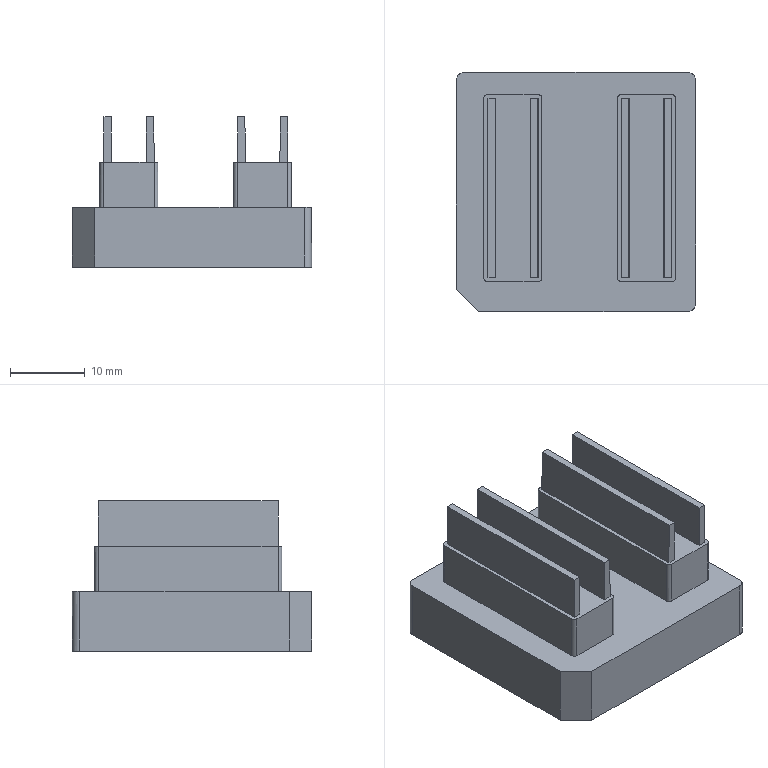NC program | PowerMill | posted with a generic post | part box 32 x 32 x 20.109 mm
Lines 1 to 1024 of 124326:
%
O0001
N104 ( POWERMILL CB  : 2026004.0)
N105 ( POST VER      : 2026.0.0.5161)
N106 ( OPTION FILE   : FANUC)
N107 ( OUTPUT WORKPLANE : WORLD)
N108 (  )
N109 ( TOOL LIST )
N110 (---------------------------------------)
N111 ( NO. | ID        | DIA.| TIP RAD|LENGTH)
N112 (---------------------------------------)
N113 (    1|D10C_1_1_1 |10.0 |  0.0   |75.56 )
N114 (   10|D3_1_1     | 3.0 |  0.0   |67.28 )
N115 (    3|D10_1_1_1  |10.0 |  0.0   |75.28 )
N116 (   10|D3_2_1     | 3.0 |  0.0   |61.32 )
N117 (   13|TEXT_D4_1_1| 4.0 |  0.3   |67.36 )
N118 (---------------------------------------)
N119 (  )
N120 ( NUMBER OF TOOLPATHS: 11.0 )
N121 ( ESTIMATED PROGRAM DURATION: 0 HOURS 28 MIN 3 SEC)
N122 (  )
N123 G00 G21 G80 G40 G17
N124 G90
N125 G54
N126 G53 Z0.0
N127 (---------------)
N128 ( START TOOLPATH : 精公开粗01-扫面平行-D10C )
N129 (---------------)
N130 ( TOOL NO.    :1 )
N131 ( TOOL TYPE   : ENDMILL)
N132 ( TOOL ID     : D10C_1_1_1)
N133 ( TOOL DIA    : 10.0 LENGTH 75.56)
N134 T1
N135 M6
N136 S8000 M03
N137 G00 G90 X0.0 Y0.0
N138 G43 Z10.2 H1
N139
N140 G05 P10000 R4
N141 X23.78 Y18.78
N142 Z1.129
N143 G01 Z-0.071 F6000.0
N144 X18.78 F10000.0
N145 X-18.78
N146 Y13.4143
N147 X18.78
N148 Y8.0486
N149 X-18.78
N150 Y2.6829
N151 X18.78
N152 Y-2.6829
N153 X-18.78
N154 Y-8.0486
N155 X18.78
N156 Y-13.4143
N157 X-18.78
N158 Y-18.78
N159 X18.78
N160 X23.78
N161 G00 Z10.2
N162 G05 P0
N163 (---------------)
N164 ( END TOOLPATH : 精公开粗01-扫面平行-D10C )
N165 (---------------)
N166 ( START TOOLPATH : 精公开粗01-外形偏置-D10C )
N167 (---------------)
N168 G00 X0.5 Y0.5 Z9.879
N169 G05 P10000 R4
N170 X1.5532 Y26.066
N171 Z0.7009
N172 G01 Z-0.4991 F6000.0
N173 Y25.5385 F10000.0
N174 G03 X6.3007 Y20.791 I4.7475 J0.0
N175 G01 X20.109
N176 G02 X21.109 Y19.791 I0.0 J-1.0
N177 G01 Y-18.791
N178 G02 X20.109 Y-19.791 I-1.0 J0.0
N179 G01 X-19.109
N180 G02 X-20.109 Y-18.791 I0.0 J1.0
N181 G01 Y19.791
N182 G02 X-19.109 Y20.791 I1.0 J0.0
N183 G01 X6.3007
N184 Y17.7935
N185 X7.0741
N186 X7.8476 Y17.7374
N187 X8.621 Y17.5636
N188 X9.2558 Y17.3098
N189 G03 X9.6337 Y17.3126 I0.1856 J0.4643
N190 G01 X10.1205 Y17.5154
N191 X10.9413 Y17.7207
N192 X11.7147 Y17.7926
N193 X13.2615 Y17.7714
N194 X14.035 Y17.642
N195 X14.8084 Y17.388
N196 X15.5818 Y16.9875
N197 X15.9412 Y16.742
N198 X16.3552 Y16.3946
N199 X16.7718 Y15.9685
N200 X17.1287 Y15.5052
N201 X17.3274 Y15.1951
N202 X17.7023 Y14.4217
N203 X17.9021 Y13.7916
N204 X18.0463 Y12.8748
N205 X18.0563 Y12.1014
N206 Y-11.1014
N207 X18.0463 Y-11.8748
N208 X17.9352 Y-12.6483
N209 X17.7023 Y-13.4217
N210 X17.3274 Y-14.1951
N211 X17.1287 Y-14.5064
N212 X16.7718 Y-14.9685
N213 X16.3552 Y-15.3962
N214 X15.9412 Y-15.742
N215 X15.5818 Y-15.9875
N216 X14.8084 Y-16.3878
N217 X14.467 Y-16.5154
N218 X14.035 Y-16.6418
N219 X13.2615 Y-16.7714
N220 X11.7147 Y-16.7926
N221 X10.9413 Y-16.7185
N222 X10.1678 Y-16.5302
N223 X9.6371 Y-16.3125
N224 G03 X9.2557 Y-16.3133 I-0.1897 J-0.4626
N225 G01 X8.7689 Y-16.5154
N226 X7.8476 Y-16.7374
N227 X7.0741 Y-16.7935
N228 X6.3007
N229 X5.5273 Y-16.7596
N230 X4.7538 Y-16.6157
N231 X4.422 Y-16.5154
N232 X3.9804 Y-16.3439
N233 X3.207 Y-15.9183
N234 X2.9505 Y-15.742
N235 X2.4336 Y-15.3013
N236 X2.1225 Y-14.9685
N237 X1.6601 Y-14.3516
N238 X1.1893 Y-13.4217
N239 X0.9577 Y-12.6483
N240 X0.8867 Y-12.2714
N241 X0.8468 Y-11.8748
N242 X0.832 Y-11.1014
N243 Y12.1014
N244 X0.8341 Y12.2088
N245 X0.1665 Y12.1981
N246 X0.168 Y12.1014
N247 Y-11.1014
N248 X0.1556 Y-11.8748
N249 X0.0443 Y-12.6483
N250 X-0.1889 Y-13.4217
N251 X-0.5637 Y-14.1951
N252 X-1.1194 Y-14.9685
N253 X-1.4336 Y-15.3013
N254 X-1.9524 Y-15.742
N255 X-2.207 Y-15.9183
N256 X-2.9804 Y-16.3439
N257 X-3.421 Y-16.5154
N258 X-3.7538 Y-16.6157
N259 X-4.5273 Y-16.7596
N260 X-5.3007 Y-16.7935
N261 X-6.0741
N262 X-6.8476 Y-16.7374
N263 X-7.621 Y-16.5636
N264 X-8.2575 Y-16.3091
N265 G03 X-8.6329 Y-16.3108 I-0.1857 J-0.4643
N266 G01 X-9.1678 Y-16.5302
N267 X-9.9413 Y-16.7185
N268 X-10.7147 Y-16.7926
N269 X-12.2615 Y-16.7714
N270 X-13.035 Y-16.6418
N271 X-13.47 Y-16.5154
N272 X-13.8084 Y-16.3878
N273 X-14.5818 Y-15.9875
N274 X-14.9391 Y-15.742
N275 X-15.3552 Y-15.3962
N276 X-15.7706 Y-14.9685
N277 X-16.1287 Y-14.5064
N278 X-16.3274 Y-14.1951
N279 X-16.7019 Y-13.4217
N280 X-16.9021 Y-12.7918
N281 X-17.0464 Y-11.8748
N282 X-17.059 Y-11.1014
N283 Y12.1014
N284 X-17.0464 Y12.8748
N285 X-16.9352 Y13.6483
N286 X-16.7019 Y14.4217
N287 X-16.3274 Y15.1951
N288 X-16.1287 Y15.5052
N289 X-15.7706 Y15.9685
N290 X-15.3552 Y16.3946
N291 X-14.9391 Y16.742
N292 X-14.5818 Y16.9875
N293 X-13.8084 Y17.388
N294 X-13.47 Y17.5154
N295 X-13.035 Y17.642
N296 X-12.2615 Y17.7714
N297 X-10.7147 Y17.7926
N298 X-9.9413 Y17.7207
N299 X-9.1678 Y17.5302
N300 X-8.6369 Y17.3124
N301 G03 X-8.2556 Y17.3131 I0.1898 J0.4626
N302 G01 X-7.7679 Y17.5154
N303 X-6.8476 Y17.7374
N304 X-6.0741 Y17.7935
N305 X-5.3007
N306 X-4.5273 Y17.7596
N307 X-3.7538 Y17.6157
N308 X-3.421 Y17.5154
N309 X-2.9804 Y17.343
N310 X-2.207 Y16.9225
N311 X-1.9525 Y16.742
N312 X-1.4336 Y16.2981
N313 X-1.1194 Y15.9685
N314 X-0.5637 Y15.1951
N315 X-0.1889 Y14.4217
N316 X0.0443 Y13.6483
N317 X0.1556 Y12.8748
N318 X0.1665 Y12.1981
N319 X0.8341 Y12.2088
N320 X0.8468 Y12.8748
N321 X0.8867 Y13.2713
N322 X0.9577 Y13.6483
N323 X1.1893 Y14.4217
N324 X1.5642 Y15.1951
N325 X2.1225 Y15.9685
N326 X2.4336 Y16.2981
N327 X2.9505 Y16.742
N328 X3.207 Y16.9225
N329 X3.9804 Y17.343
N330 X4.422 Y17.5154
N331 X4.7538 Y17.6157
N332 X5.5273 Y17.7596
N333 X6.3007 Y17.7935
N334 Y20.791
N335 G00 Z3.3228
N336 G01 X1.5532 Y26.066
N337 G00 Z0.3228
N338 G01 Z-0.8772 F6000.0
N339 Y25.5385 F10000.0
N340 G03 X6.3007 Y20.791 I4.7475 J0.0
N341 G01 X20.109
N342 G02 X21.109 Y19.791 I0.0 J-1.0
N343 G01 Y-18.791
N344 G02 X20.109 Y-19.791 I-1.0 J0.0
N345 G01 X-19.109
N346 G02 X-20.109 Y-18.791 I0.0 J1.0
N347 G01 Y19.791
N348 G02 X-19.109 Y20.791 I1.0 J0.0
N349 G01 X6.3007
N350 Y17.7935
N351 X7.0741
N352 X7.8476 Y17.7379
N353 X8.621 Y17.5646
N354 X9.2575 Y17.3106
N355 G03 X9.6328 Y17.3125 I0.1853 J0.4644
N356 G01 X9.6987 Y17.3396
N357 X10.1205 Y17.5153
N358 X10.1358 Y17.5192
N359 X10.1678 Y17.5323
N360 X10.9413 Y17.7219
N361 X11.7147 Y17.7927
N362 X13.2615 Y17.7717
N363 X14.035 Y17.6428
N364 X14.4735 Y17.5154
N365 X14.8084 Y17.3894
N366 X15.5818 Y16.9901
N367 X15.9445 Y16.742
N368 X16.3552 Y16.4012
N369 X16.7751 Y15.9685
N370 X17.1287 Y15.5116
N371 X17.3308 Y15.1951
N372 X17.7056 Y14.4217
N373 X17.9021 Y13.8045
N374 X18.0501 Y12.8748
N375 X18.0615 Y12.1014
N376 Y-11.1014
N377 X18.0501 Y-11.8748
N378 X17.9391 Y-12.6483
N379 X17.7056 Y-13.4217
N380 X17.3308 Y-14.1951
N381 X17.1287 Y-14.5116
N382 X16.7751 Y-14.9685
N383 X16.3552 Y-15.4005
N384 X15.9445 Y-15.742
N385 X15.5818 Y-15.9901
N386 X14.8084 Y-16.3894
N387 X14.4735 Y-16.5154
N388 X14.035 Y-16.6428
N389 X13.2615 Y-16.7717
N390 X11.7147 Y-16.7927
N391 X10.9413 Y-16.7215
N392 X10.1678 Y-16.5323
N393 X9.6375 Y-16.3145
N394 G03 X9.2555 Y-16.3153 I-0.19 J-0.4625
N395 G01 X8.7743 Y-16.5154
N396 X7.8476 Y-16.7379
N397 X7.0741 Y-16.7935
N398 X6.3007
N399 X5.5273 Y-16.761
N400 X4.7538 Y-16.6167
N401 X4.4177 Y-16.5154
N402 X3.9804 Y-16.3456
N403 X3.207 Y-15.9247
N404 X2.9467 Y-15.742
N405 X2.4336 Y-15.3045
N406 X2.1164 Y-14.9685
N407 X1.971 Y-14.7662
N408 X1.6602 Y-14.3516
N409 X1.63 Y-14.292
N410 X1.5604 Y-14.1951
N411 X1.1856 Y-13.4217
N412 X0.9531 Y-12.6483
N413 X0.8867 Y-12.294
N414 X0.842 Y-11.8748
N415 X0.8287 Y-11.1014
N416 Y12.1014
N417 X0.1713
N418 Y-11.1014
N419 X0.1589 Y-11.8748
N420 X0.0479 Y-12.6483
N421 X-0.1856 Y-13.4217
N422 X-0.5604 Y-14.1951
N423 X-1.1161 Y-14.9685
N424 X-1.4336 Y-15.3045
N425 X-1.9476 Y-15.742
N426 X-2.207 Y-15.9247
N427 X-2.9804 Y-16.3456
N428 X-3.4177 Y-16.5154
N429 X-3.7538 Y-16.6167
N430 X-4.5273 Y-16.761
N431 X-5.3007 Y-16.7935
N432 X-6.0741
N433 X-6.8476 Y-16.7379
N434 X-7.621 Y-16.5646
N435 X-8.2575 Y-16.3106
N436 G03 X-8.6328 Y-16.3125 I-0.1853 J-0.4644
N437 G01 X-9.1678 Y-16.5323
N438 X-9.9413 Y-16.7215
N439 X-10.7147 Y-16.7927
N440 X-12.2615 Y-16.7717
N441 X-13.035 Y-16.6428
N442 X-13.4735 Y-16.5154
N443 X-13.8084 Y-16.3894
N444 X-14.5818 Y-15.9901
N445 X-14.9445 Y-15.742
N446 X-15.3552 Y-15.4005
N447 X-15.7751 Y-14.9685
N448 X-16.1287 Y-14.5116
N449 X-16.3308 Y-14.1951
N450 X-16.7056 Y-13.4217
N451 X-16.9021 Y-12.8046
N452 X-17.0501 Y-11.8748
N453 X-17.0625 Y-11.1014
N454 Y12.1014
N455 X-17.0501 Y12.8748
N456 X-16.9391 Y13.6483
N457 X-16.7056 Y14.4217
N458 X-16.3308 Y15.1951
N459 X-16.1287 Y15.5116
N460 X-15.7751 Y15.9685
N461 X-15.3552 Y16.4012
N462 X-14.9445 Y16.742
N463 X-14.5818 Y16.9901
N464 X-13.8084 Y17.3894
N465 X-13.4735 Y17.5154
N466 X-13.035 Y17.6428
N467 X-12.2615 Y17.7717
N468 X-10.7147 Y17.7927
N469 X-9.9413 Y17.7219
N470 X-9.1678 Y17.5323
N471 X-8.6375 Y17.3144
N472 G03 X-8.2555 Y17.3153 I0.19 J0.4625
N473 G01 X-7.7743 Y17.5154
N474 X-6.8476 Y17.7379
N475 X-6.0741 Y17.7935
N476 X-5.3007
N477 X-4.5273 Y17.761
N478 X-3.7538 Y17.6167
N479 X-3.4177 Y17.5154
N480 X-2.9804 Y17.3456
N481 X-2.207 Y16.9247
N482 X-1.9476 Y16.742
N483 X-1.4336 Y16.3045
N484 X-1.1161 Y15.9685
N485 X-0.5604 Y15.1951
N486 X-0.1856 Y14.4217
N487 X0.0479 Y13.6483
N488 X0.1589 Y12.8748
N489 X0.1713 Y12.1014
N490 X0.8287
N491 X0.842 Y12.8748
N492 X0.8867 Y13.293
N493 X0.9531 Y13.6483
N494 X1.1856 Y14.4217
N495 X1.5604 Y15.1951
N496 X2.1164 Y15.9685
N497 X2.4336 Y16.3045
N498 X2.9467 Y16.742
N499 X3.207 Y16.9247
N500 X3.9804 Y17.3456
N501 X4.4177 Y17.5154
N502 X4.7538 Y17.6167
N503 X5.5273 Y17.761
N504 X6.3007 Y17.7935
N505 Y20.791
N506 G00 Z2.9447
N507 G01 X1.5532 Y26.066
N508 G00 Z-0.0553
N509 G01 Z-1.2553 F6000.0
N510 Y25.5385 F10000.0
N511 G03 X6.3007 Y20.791 I4.7475 J0.0
N512 G01 X20.109
N513 G02 X21.109 Y19.791 I0.0 J-1.0
N514 G01 Y-18.791
N515 G02 X20.109 Y-19.791 I-1.0 J0.0
N516 G01 X-19.109
N517 G02 X-20.109 Y-18.791 I0.0 J1.0
N518 G01 Y19.791
N519 G02 X-19.109 Y20.791 I1.0 J0.0
N520 G01 X6.3007
N521 Y17.7935
N522 X7.0741
N523 X7.8476 Y17.7384
N524 X8.621 Y17.5656
N525 X9.2577 Y17.3121
N526 G03 X9.6323 Y17.3139 I0.185 J0.4645
N527 G01 X9.9334 Y17.4373
N528 X10.1205 Y17.5153
N529 X10.1286 Y17.5173
N530 X10.1678 Y17.5334
N531 X10.9413 Y17.7224
N532 X11.7147 Y17.7927
N533 X13.2615 Y17.772
N534 X14.035 Y17.6436
N535 X14.4768 Y17.5154
N536 X14.8084 Y17.3907
N537 X15.5818 Y16.9924
N538 X15.9478 Y16.742
N539 X16.3552 Y16.4042
N540 X16.7784 Y15.9685
N541 X17.1287 Y15.5165
N542 X17.3341 Y15.1951
N543 X17.7089 Y14.4217
N544 X17.9021 Y13.8173
N545 X18.0534 Y12.8748
N546 X18.0658 Y12.1014
N547 Y-11.1014
N548 X18.0534 Y-11.8748
N549 X17.9424 Y-12.6483
N550 X17.7089 Y-13.4217
N551 X17.3341 Y-14.1951
N552 X17.1287 Y-14.5165
N553 X16.7784 Y-14.9685
N554 X16.3552 Y-15.4042
N555 X15.9478 Y-15.742
N556 X15.5818 Y-15.9924
N557 X14.8084 Y-16.3907
N558 X14.4768 Y-16.5154
N559 X14.035 Y-16.6436
N560 X13.2615 Y-16.772
N561 X11.7147 Y-16.7927
N562 X10.9413 Y-16.7224
N563 X10.1678 Y-16.5334
N564 X9.637 Y-16.3157
N565 G03 X9.2553 Y-16.3167 I-0.1897 J-0.4627
N566 G01 X8.7776 Y-16.5154
N567 X7.8476 Y-16.7384
N568 X7.0741 Y-16.7935
N569 X6.3007
N570 X5.5273 Y-16.7617
N571 X4.7538 Y-16.6176
N572 X4.4144 Y-16.5154
N573 X3.9804 Y-16.347
N574 X3.207 Y-15.9268
N575 X2.9434 Y-15.742
N576 X2.4336 Y-15.3077
N577 X2.1128 Y-14.9685
N578 X1.8834 Y-14.6494
N579 X1.6602 Y-14.3516
N580 X1.6382 Y-14.308
N581 X1.5571 Y-14.1951
N582 X1.1823 Y-13.4217
N583 X0.9488 Y-12.6483
N584 X0.9345 Y-12.5485
N585 X0.8868 Y-12.294
N586 X0.8544 Y-11.991
N587 X0.8378 Y-11.8748
N588 X0.8254 Y-11.1014
N589 Y12.1014
N590 X0.1746
N591 Y-11.1014
N592 X0.1622 Y-11.8748
N593 X0.0512 Y-12.6483
N594 X-0.1823 Y-13.4217
N595 X-0.5571 Y-14.1951
N596 X-1.1128 Y-14.9685
N597 X-1.4336 Y-15.3077
N598 X-1.9434 Y-15.742
N599 X-2.207 Y-15.9268
N600 X-2.9804 Y-16.347
N601 X-3.4144 Y-16.5154
N602 X-3.7538 Y-16.6176
N603 X-4.5273 Y-16.7617
N604 X-5.3007 Y-16.7935
N605 X-6.0741
N606 X-6.8476 Y-16.7384
N607 X-7.621 Y-16.5656
N608 X-8.2577 Y-16.3121
N609 G03 X-8.6322 Y-16.3139 I-0.185 J-0.4645
N610 G01 X-9.1678 Y-16.5334
N611 X-9.9413 Y-16.7224
N612 X-10.7147 Y-16.7927
N613 X-12.2615 Y-16.772
N614 X-13.035 Y-16.6436
N615 X-13.4768 Y-16.5154
N616 X-13.8084 Y-16.3907
N617 X-14.5818 Y-15.9924
N618 X-14.9478 Y-15.742
N619 X-15.3552 Y-15.4042
N620 X-15.7784 Y-14.9685
N621 X-16.1287 Y-14.5165
N622 X-16.3341 Y-14.1951
N623 X-16.7089 Y-13.4217
N624 X-16.9021 Y-12.8174
N625 X-17.0534 Y-11.8748
N626 X-17.0658 Y-11.1014
N627 Y12.1014
N628 X-17.0534 Y12.8748
N629 X-16.9424 Y13.6483
N630 X-16.7089 Y14.4217
N631 X-16.3341 Y15.1951
N632 X-16.1287 Y15.5165
N633 X-15.7784 Y15.9685
N634 X-15.3552 Y16.4042
N635 X-14.9478 Y16.742
N636 X-14.5818 Y16.9924
N637 X-13.8084 Y17.3907
N638 X-13.4768 Y17.5154
N639 X-13.035 Y17.6436
N640 X-12.2615 Y17.772
N641 X-10.7147 Y17.7927
N642 X-9.9413 Y17.7224
N643 X-9.1678 Y17.5334
N644 X-8.6371 Y17.3158
N645 G03 X-8.2554 Y17.3167 I0.1897 J0.4626
N646 G01 X-7.7776 Y17.5154
N647 X-6.8476 Y17.7384
N648 X-6.0741 Y17.7935
N649 X-5.3007
N650 X-4.5273 Y17.7617
N651 X-3.7538 Y17.6176
N652 X-3.4144 Y17.5154
N653 X-2.9804 Y17.347
N654 X-2.207 Y16.9268
N655 X-1.9434 Y16.742
N656 X-1.4336 Y16.3077
N657 X-1.1128 Y15.9685
N658 X-0.5571 Y15.1951
N659 X-0.1823 Y14.4217
N660 X0.0512 Y13.6483
N661 X0.1622 Y12.8748
N662 X0.1746 Y12.1014
N663 X0.8254
N664 X0.8378 Y12.8748
N665 X0.8546 Y12.9918
N666 X0.8868 Y13.293
N667 X0.9343 Y13.5473
N668 X0.9488 Y13.6483
N669 X1.1823 Y14.4217
N670 X1.5571 Y15.1951
N671 X2.1128 Y15.9685
N672 X2.4336 Y16.3077
N673 X2.9434 Y16.742
N674 X3.207 Y16.9268
N675 X3.9804 Y17.347
N676 X4.4144 Y17.5154
N677 X4.7538 Y17.6176
N678 X5.5273 Y17.7617
N679 X6.3007 Y17.7935
N680 Y20.791
N681 G00 Z2.5666
N682 G01 X1.5532 Y26.066
N683 G00 Z-0.4334
N684 G01 Z-1.6334 F6000.0
N685 Y25.5385 F10000.0
N686 G03 X6.3007 Y20.791 I4.7475 J0.0
N687 G01 X20.109
N688 G02 X21.109 Y19.791 I0.0 J-1.0
N689 G01 Y-18.791
N690 G02 X20.109 Y-19.791 I-1.0 J0.0
N691 G01 X-19.109
N692 G02 X-20.109 Y-18.791 I0.0 J1.0
N693 G01 Y19.791
N694 G02 X-19.109 Y20.791 I1.0 J0.0
N695 G01 X6.3007
N696 Y17.7935
N697 X7.0741
N698 X7.8476 Y17.7389
N699 X8.621 Y17.5666
N700 X9.2578 Y17.3135
N701 G03 X9.6317 Y17.3153 I0.1847 J0.4647
N702 G01 X10.1074 Y17.5098
N703 X10.1205 Y17.5152
N704 X10.1212 Y17.5154
N705 X10.1678 Y17.5345
N706 X10.9413 Y17.723
N707 X11.7147 Y17.7928
N708 X13.2615 Y17.7723
N709 X14.035 Y17.6444
N710 X14.4801 Y17.5154
N711 X14.8084 Y17.3921
N712 X15.5818 Y16.9945
N713 X15.9511 Y16.742
N714 X16.3552 Y16.4072
N715 X16.7817 Y15.9685
N716 X17.1287 Y15.5212
N717 X17.3374 Y15.1951
N718 X17.7122 Y14.4217
N719 X17.9021 Y13.8302
N720 X18.0567 Y12.8748
N721 X18.0691 Y12.1014
N722 Y-11.1014
N723 X18.0567 Y-11.8748
N724 X17.9457 Y-12.6483
N725 X17.7122 Y-13.4217
N726 X17.3374 Y-14.1951
N727 X17.1287 Y-14.5212
N728 X16.7817 Y-14.9685
N729 X16.3552 Y-15.4072
N730 X15.9511 Y-15.742
N731 X15.5818 Y-15.9945
N732 X14.8084 Y-16.3921
N733 X14.4801 Y-16.5154
N734 X14.035 Y-16.6444
N735 X13.2615 Y-16.7723
N736 X11.7147 Y-16.7928
N737 X10.9413 Y-16.723
N738 X10.1678 Y-16.5345
N739 X9.6366 Y-16.3171
N740 G03 X9.2552 Y-16.3181 I-0.1894 J-0.4627
N741 G01 X8.7809 Y-16.5154
N742 X7.8476 Y-16.7389
N743 X7.0741 Y-16.7935
N744 X6.3007
N745 X5.5273 Y-16.7621
N746 X4.7538 Y-16.6185
N747 X4.4111 Y-16.5154
N748 X3.9804 Y-16.3485
N749 X3.207 Y-15.929
N750 X2.9401 Y-15.742
N751 X2.4336 Y-15.3109
N752 X2.1095 Y-14.9685
N753 X1.8023 Y-14.541
N754 X1.6603 Y-14.3515
N755 X1.6462 Y-14.3238
N756 X1.5538 Y-14.1951
N757 X1.179 Y-13.4217
N758 X0.9455 Y-12.6483
N759 X0.9202 Y-12.4722
N760 X0.8868 Y-12.294
N761 X0.8642 Y-12.0819
N762 X0.8345 Y-11.8748
N763 X0.8221 Y-11.1014
N764 Y12.1014
N765 X0.1779
N766 Y-11.1014
N767 X0.1655 Y-11.8748
N768 X0.0545 Y-12.6483
N769 X-0.179 Y-13.4217
N770 X-0.5538 Y-14.1951
N771 X-1.1095 Y-14.9685
N772 X-1.4336 Y-15.3109
N773 X-1.9401 Y-15.742
N774 X-2.207 Y-15.929
N775 X-2.9804 Y-16.3485
N776 X-3.4111 Y-16.5154
N777 X-3.7538 Y-16.6185
N778 X-4.5273 Y-16.7621
N779 X-5.3007 Y-16.7935
N780 X-6.0741
N781 X-6.8476 Y-16.7389
N782 X-7.621 Y-16.5666
N783 X-8.2579 Y-16.3135
N784 G03 X-8.6317 Y-16.3153 I-0.1846 J-0.4647
N785 G01 X-9.1678 Y-16.5345
N786 X-9.9413 Y-16.723
N787 X-10.7147 Y-16.7928
N788 X-12.2615 Y-16.7723
N789 X-13.035 Y-16.6444
N790 X-13.4801 Y-16.5154
N791 X-13.8084 Y-16.3921
N792 X-14.5818 Y-15.9945
N793 X-14.9511 Y-15.742
N794 X-15.3552 Y-15.4072
N795 X-15.7817 Y-14.9685
N796 X-16.1287 Y-14.5212
N797 X-16.3374 Y-14.1951
N798 X-16.7122 Y-13.4217
N799 X-16.9021 Y-12.8302
N800 X-17.0567 Y-11.8748
N801 X-17.0691 Y-11.1014
N802 Y12.1014
N803 X-17.0567 Y12.8748
N804 X-16.9457 Y13.6483
N805 X-16.7122 Y14.4217
N806 X-16.3374 Y15.1951
N807 X-16.1287 Y15.5212
N808 X-15.7817 Y15.9685
N809 X-15.3552 Y16.4072
N810 X-14.9511 Y16.742
N811 X-14.5818 Y16.9945
N812 X-13.8084 Y17.3921
N813 X-13.4801 Y17.5154
N814 X-13.035 Y17.6444
N815 X-12.2615 Y17.7723
N816 X-10.7147 Y17.7928
N817 X-9.9413 Y17.723
N818 X-9.1678 Y17.5345
N819 X-8.6366 Y17.317
N820 G03 X-8.2552 Y17.3181 I0.1894 J0.4628
N821 G01 X-7.7809 Y17.5154
N822 X-6.8476 Y17.7389
N823 X-6.0741 Y17.7935
N824 X-5.3007
N825 X-4.5273 Y17.7621
N826 X-3.7538 Y17.6185
N827 X-3.4111 Y17.5154
N828 X-2.9804 Y17.3485
N829 X-2.207 Y16.929
N830 X-1.9401 Y16.742
N831 X-1.4336 Y16.3109
N832 X-1.1095 Y15.9685
N833 X-0.5538 Y15.1951
N834 X-0.179 Y14.4217
N835 X0.0545 Y13.6483
N836 X0.1655 Y12.8748
N837 X0.1779 Y12.1014
N838 X0.8221
N839 X0.8345 Y12.8748
N840 X0.8644 Y13.0833
N841 X0.8868 Y13.293
N842 X0.9199 Y13.47
N843 X0.9455 Y13.6483
N844 X1.179 Y14.4217
N845 X1.5538 Y15.1951
N846 X2.1095 Y15.9685
N847 X2.4336 Y16.3109
N848 X2.9401 Y16.742
N849 X3.207 Y16.929
N850 X3.9804 Y17.3485
N851 X4.4111 Y17.5154
N852 X4.7538 Y17.6185
N853 X5.5273 Y17.7621
N854 X6.3007 Y17.7935
N855 Y20.791
N856 G00 Z2.1885
N857 G01 X1.5532 Y26.066
N858 G00 Z-0.8115
N859 G01 Z-2.0115 F6000.0
N860 Y25.5385 F10000.0
N861 G03 X6.3007 Y20.791 I4.7475 J0.0
N862 G01 X20.109
N863 G02 X21.109 Y19.791 I0.0 J-1.0
N864 G01 Y-18.791
N865 G02 X20.109 Y-19.791 I-1.0 J0.0
N866 G01 X-19.109
N867 G02 X-20.109 Y-18.791 I0.0 J1.0
N868 G01 Y19.791
N869 G02 X-19.109 Y20.791 I1.0 J0.0
N870 G01 X6.3007
N871 Y17.7935
N872 X7.0741
N873 X7.8476 Y17.7393
N874 X8.621 Y17.5676
N875 X9.2568 Y17.3154
N876 G03 X9.6329 Y17.3185 I0.1843 J0.4648
N877 G01 X10.107 Y17.5154
N878 X10.1436 Y17.5245
N879 X10.1678 Y17.5344
N880 X10.8381 Y17.6978
N881 X10.9413 Y17.7235
N882 X11.7147 Y17.7928
N883 X13.2615 Y17.7726
N884 X14.035 Y17.6452
N885 X14.4834 Y17.5154
N886 X14.8084 Y17.3935
N887 X15.5818 Y16.9965
N888 X15.9544 Y16.742
N889 X16.3552 Y16.4102
N890 X16.785 Y15.9685
N891 X17.1287 Y15.526
N892 X17.3407 Y15.1951
N893 X17.7155 Y14.4217
N894 X17.9021 Y13.843
N895 X18.06 Y12.8748
N896 X18.0724 Y12.1014
N897 Y-11.1014
N898 X18.06 Y-11.8748
N899 X17.949 Y-12.6483
N900 X17.7155 Y-13.4217
N901 X17.3407 Y-14.1951
N902 X17.1287 Y-14.526
N903 X16.785 Y-14.9685
N904 X16.3552 Y-15.4102
N905 X15.9544 Y-15.742
N906 X15.5818 Y-15.9965
N907 X14.8084 Y-16.3935
N908 X14.4834 Y-16.5154
N909 X14.035 Y-16.6452
N910 X13.2615 Y-16.7726
N911 X11.7147 Y-16.7928
N912 X10.9413 Y-16.7235
N913 X10.1678 Y-16.5355
N914 X9.6367 Y-16.3186
N915 G03 X9.256 Y-16.3196 I-0.1891 J-0.4629
N916 G01 X8.7842 Y-16.5154
N917 X7.8476 Y-16.7393
N918 X7.0741 Y-16.7935
N919 X6.3007
N920 X5.5273 Y-16.7625
N921 X4.7538 Y-16.6193
N922 X4.4078 Y-16.5154
N923 X3.9804 Y-16.3499
N924 X3.207 Y-15.9312
N925 X2.9368 Y-15.742
N926 X2.4336 Y-15.3141
N927 X2.1062 Y-14.9685
N928 X1.7211 Y-14.4326
N929 X1.6603 Y-14.3515
N930 X1.6543 Y-14.3396
N931 X1.5505 Y-14.1951
N932 X1.1757 Y-13.4217
N933 X0.9422 Y-12.6483
N934 X0.9059 Y-12.3958
N935 X0.8869 Y-12.294
N936 X0.8739 Y-12.1728
N937 X0.8312 Y-11.8748
N938 X0.8188 Y-11.1014
N939 Y12.1014
N940 X0.1812
N941 Y-11.1014
N942 X0.1688 Y-11.8748
N943 X0.0578 Y-12.6483
N944 X-0.1757 Y-13.4217
N945 X-0.5505 Y-14.1951
N946 X-1.1062 Y-14.9685
N947 X-1.4336 Y-15.3141
N948 X-1.9368 Y-15.742
N949 X-2.207 Y-15.9312
N950 X-2.9804 Y-16.3499
N951 X-3.4078 Y-16.5154
N952 X-3.7538 Y-16.6193
N953 X-4.5273 Y-16.7625
N954 X-5.3007 Y-16.7935
N955 X-6.0741
N956 X-6.8476 Y-16.7393
N957 X-7.621 Y-16.5676
N958 X-8.2567 Y-16.3154
N959 G03 X-8.6329 Y-16.3185 I-0.1844 J-0.4648
N960 G01 X-9.107 Y-16.5154
N961 X-9.1436 Y-16.5245
N962 X-9.1678 Y-16.5344
N963 X-9.8375 Y-16.6976
N964 X-9.9413 Y-16.7235
N965 X-10.7147 Y-16.7928
N966 X-12.2615 Y-16.7726
N967 X-13.035 Y-16.6452
N968 X-13.4834 Y-16.5154
N969 X-13.8084 Y-16.3935
N970 X-14.5818 Y-15.9965
N971 X-14.9544 Y-15.742
N972 X-15.3552 Y-15.4102
N973 X-15.785 Y-14.9685
N974 X-16.1287 Y-14.526
N975 X-16.3407 Y-14.1951
N976 X-16.7155 Y-13.4217
N977 X-16.9021 Y-12.8431
N978 X-17.06 Y-11.8748
N979 X-17.0724 Y-11.1014
N980 Y12.1014
N981 X-17.06 Y12.8748
N982 X-16.949 Y13.6483
N983 X-16.7155 Y14.4217
N984 X-16.3407 Y15.1951
N985 X-16.1287 Y15.526
N986 X-15.785 Y15.9685
N987 X-15.3552 Y16.4102
N988 X-14.9544 Y16.742
N989 X-14.5818 Y16.9965
N990 X-13.8084 Y17.3935
N991 X-13.4834 Y17.5154
N992 X-13.035 Y17.6452
N993 X-12.2615 Y17.7726
N994 X-10.7147 Y17.7928
N995 X-9.9413 Y17.7235
N996 X-9.1678 Y17.5355
N997 X-8.6367 Y17.3186
N998 G03 X-8.2561 Y17.3197 I0.189 J0.4629
N999 G01 X-7.7842 Y17.5154
N1000 X-6.8476 Y17.7393
N1001 X-6.0741 Y17.7935
N1002 X-5.3007
N1003 X-4.5273 Y17.7625
N1004 X-3.7538 Y17.6193
N1005 X-3.4078 Y17.5154
N1006 X-2.9804 Y17.3499
N1007 X-2.207 Y16.9312
N1008 X-1.9368 Y16.742
N1009 X-1.4336 Y16.3141
N1010 X-1.1062 Y15.9685
N1011 X-0.5505 Y15.1951
N1012 X-0.1757 Y14.4217
N1013 X0.0578 Y13.6483
N1014 X0.1688 Y12.8748
N1015 X0.1812 Y12.1014
N1016 X0.8188
N1017 X0.8312 Y12.8748
N1018 X0.8742 Y13.1748
N1019 X0.8869 Y13.293
N1020 X0.9055 Y13.3927
N1021 X0.9422 Y13.6483
N1022 X1.1757 Y14.4217
N1023 X1.5505 Y15.1951
N1024 X2.1062 Y15.9685
N1025 X2.4336 Y16.3141
N1026 X2.9368 Y16.742
N1027 X3.207 Y16.9312
N1028 X3.9804 Y17.3499
N1029 X4.4078 Y17.5154
N1030 X4.7538 Y17.6193
N1031 X5.5273 Y17.7625
N1032 X6.3007 Y17.7935
N1033 Y20.791
N1034 G00 Z1.8103
N1035 G01 X1.5532 Y26.066
N1036 G00 Z-1.1897
N1037 G01 Z-2.3897 F6000.0
N1038 Y25.5385 F10000.0
N1039 G03 X6.3007 Y20.791 I4.7475 J0.0
N1040 G01 X20.109
N1041 G02 X21.109 Y19.791 I0.0 J-1.0
N1042 G01 Y-18.791
N1043 G02 X20.109 Y-19.791 I-1.0 J0.0
N1044 G01 X-19.109
N1045 G02 X-20.109 Y-18.791 I0.0 J1.0
N1046 G01 Y19.791
N1047 G02 X-19.109 Y20.791 I1.0 J0.0
N1048 G01 X6.3007
N1049 Y17.7935
N1050 X7.0741
N1051 X7.8476 Y17.7398
N1052 X8.621 Y17.5686
N1053 X9.2568 Y17.3169
N1054 G03 X9.6324 Y17.3199 I0.1841 J0.4649
N1055 G01 X10.1037 Y17.5154
N1056 X10.149 Y17.5267
N1057 X10.1679 Y17.5344
N1058 X10.7219 Y17.6694
N1059 X10.9413 Y17.7241
N1060 X11.7147 Y17.7929
N1061 X13.2615 Y17.7729
N1062 X14.035 Y17.646
N1063 X14.4867 Y17.5154
N1064 X14.8084 Y17.3948
N1065 X15.5818 Y16.9986
N1066 X15.9577 Y16.742
N1067 X16.3552 Y16.4132
N1068 X16.7883 Y15.9685
N1069 X17.1287 Y15.5307
N1070 X17.344 Y15.1951
N1071 X17.7188 Y14.4217
N1072 X17.7682 Y14.2582
N1073 X17.902 Y13.843
N1074 X17.9121 Y13.7817
N1075 X17.9523 Y13.6483
N1076 X18.0633 Y12.8748
N1077 X18.0757 Y12.1014
N1078 Y-11.1014
N1079 X18.0633 Y-11.8748
N1080 X17.9523 Y-12.6483
N1081 X17.7188 Y-13.4217
N1082 X17.344 Y-14.1951
N1083 X17.1287 Y-14.5307
N1084 X16.7883 Y-14.9685
N1085 X16.3552 Y-15.4132
N1086 X15.9577 Y-15.742
N1087 X15.5818 Y-15.9986
N1088 X14.8084 Y-16.3948
N1089 X14.4867 Y-16.5154
N1090 X14.035 Y-16.646
N1091 X13.2615 Y-16.7729
N1092 X11.7147 Y-16.7929
N1093 X10.9413 Y-16.7241
N1094 X10.1678 Y-16.5366
N1095 X9.6363 Y-16.3199
N1096 G03 X9.2559 Y-16.3211 I-0.1888 J-0.463
N1097 G01 X8.7875 Y-16.5154
N1098 X7.8476 Y-16.7398
N1099 X7.0741 Y-16.7935
N1100 X6.3007
N1101 X5.5273 Y-16.7628
N1102 X4.7538 Y-16.6202
N1103 X4.4045 Y-16.5154
N1104 X3.9804 Y-16.3514
N1105 X3.207 Y-15.9333
N1106 X2.9335 Y-15.742
N1107 X2.4336 Y-15.3173
N1108 X2.1029 Y-14.9685
N1109 X1.6601 Y-14.3781
N1110 X1.5472 Y-14.1951
N1111 X1.1724 Y-13.4217
N1112 X0.9389 Y-12.6483
N1113 X0.8917 Y-12.3194
N1114 X0.8869 Y-12.294
N1115 X0.8837 Y-12.2637
N1116 X0.8279 Y-11.8748
N1117 X0.8155 Y-11.1014
N1118 Y12.1014
N1119 X0.1845
N1120 Y-11.1014
N1121 X0.1721 Y-11.8748